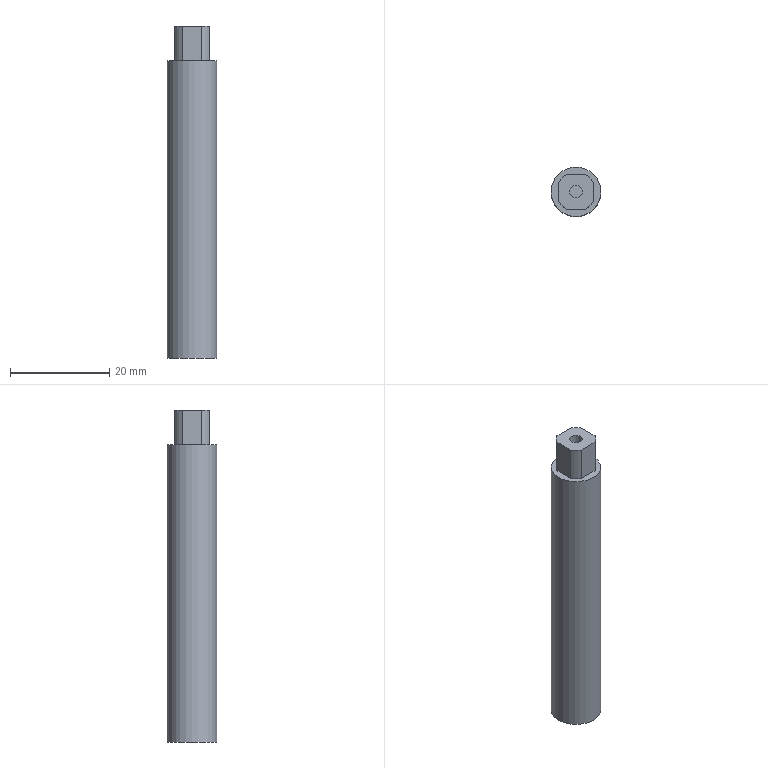Part | NX | features DATUM_CSYS 4, EXTRUDE 3, SKETCH 3 | 1 solid | 14 faces | box 10 x 10 x 67 mm | volume 4993 mm3 | plane 8 | cylinder 6 | commonest cylinder face diameters 8 x4 2.5 x1 10 x1
STEP:
#1=CARTESIAN_POINT('',(5.,0.,60.));
#2=VERTEX_POINT('',#1);
#3=CARTESIAN_POINT('',(0.,0.,60.));
#4=DIRECTION('',(0.,0.,1.));
#5=DIRECTION('',(1.,0.,0.));
#6=AXIS2_PLACEMENT_3D('',#3,#4,#5);
#7=CIRCLE('',#6,5.);
#8=EDGE_CURVE('',#2,#2,#7,.T.);
#9=ORIENTED_EDGE('',*,*,#8,.F.);
#10=EDGE_LOOP('',(#9));
#11=FACE_BOUND('',#10,.T.);
#12=CARTESIAN_POINT('',(5.,0.,0.));
#13=VERTEX_POINT('',#12);
#14=CARTESIAN_POINT('',(0.,0.,0.));
#15=DIRECTION('',(0.,0.,1.));
#16=DIRECTION('',(1.,0.,0.));
#17=AXIS2_PLACEMENT_3D('',#14,#15,#16);
#18=CIRCLE('',#17,5.);
#19=EDGE_CURVE('',#13,#13,#18,.T.);
#20=ORIENTED_EDGE('',*,*,#19,.T.);
#21=EDGE_LOOP('',(#20));
#22=FACE_BOUND('',#21,.T.);
#23=CARTESIAN_POINT('',(0.,0.,60.));
#24=DIRECTION('',(0.,0.,-1.));
#25=DIRECTION('',(-1.,0.,0.));
#26=AXIS2_PLACEMENT_3D('',#23,#24,#25);
#27=CYLINDRICAL_SURFACE('',#26,5.);
#28=ADVANCED_FACE('',(#11,#22),#27,.T.);
#29=CARTESIAN_POINT('',(-3.5,1.936,60.));
#30=VERTEX_POINT('',#29);
#31=CARTESIAN_POINT('',(-3.5,-1.936,60.));
#32=VERTEX_POINT('',#31);
#33=CARTESIAN_POINT('',(-3.5,1.936,60.));
#34=DIRECTION('',(0.,-1.,0.));
#35=VECTOR('',#34,1000.);
#36=LINE('',#33,#35);
#37=EDGE_CURVE('',#30,#32,#36,.T.);
#38=ORIENTED_EDGE('',*,*,#37,.F.);
#39=CARTESIAN_POINT('',(-1.936,3.5,60.));
#40=VERTEX_POINT('',#39);
#41=CARTESIAN_POINT('',(0.,0.,60.));
#42=DIRECTION('',(0.,0.,1.));
#43=DIRECTION('',(1.,0.,0.));
#44=AXIS2_PLACEMENT_3D('',#41,#42,#43);
#45=CIRCLE('',#44,4.);
#46=EDGE_CURVE('',#40,#30,#45,.T.);
#47=ORIENTED_EDGE('',*,*,#46,.F.);
#48=CARTESIAN_POINT('',(1.936,3.5,60.));
#49=VERTEX_POINT('',#48);
#50=CARTESIAN_POINT('',(1.936,3.5,60.));
#51=DIRECTION('',(-1.,0.,0.));
#52=VECTOR('',#51,1000.);
#53=LINE('',#50,#52);
#54=EDGE_CURVE('',#49,#40,#53,.T.);
#55=ORIENTED_EDGE('',*,*,#54,.F.);
#56=CARTESIAN_POINT('',(3.5,1.936,60.));
#57=VERTEX_POINT('',#56);
#58=CARTESIAN_POINT('',(0.,0.,60.));
#59=DIRECTION('',(0.,0.,1.));
#60=DIRECTION('',(1.,0.,0.));
#61=AXIS2_PLACEMENT_3D('',#58,#59,#60);
#62=CIRCLE('',#61,4.);
#63=EDGE_CURVE('',#57,#49,#62,.T.);
#64=ORIENTED_EDGE('',*,*,#63,.F.);
#65=CARTESIAN_POINT('',(3.5,-1.936,60.));
#66=VERTEX_POINT('',#65);
#67=CARTESIAN_POINT('',(3.5,-1.936,60.));
#68=DIRECTION('',(0.,1.,0.));
#69=VECTOR('',#68,1000.);
#70=LINE('',#67,#69);
#71=EDGE_CURVE('',#66,#57,#70,.T.);
#72=ORIENTED_EDGE('',*,*,#71,.F.);
#73=CARTESIAN_POINT('',(1.936,-3.5,60.));
#74=VERTEX_POINT('',#73);
#75=CARTESIAN_POINT('',(0.,0.,60.));
#76=DIRECTION('',(0.,0.,1.));
#77=DIRECTION('',(1.,0.,0.));
#78=AXIS2_PLACEMENT_3D('',#75,#76,#77);
#79=CIRCLE('',#78,4.);
#80=EDGE_CURVE('',#74,#66,#79,.T.);
#81=ORIENTED_EDGE('',*,*,#80,.F.);
#82=CARTESIAN_POINT('',(-1.936,-3.5,60.));
#83=VERTEX_POINT('',#82);
#84=CARTESIAN_POINT('',(-1.936,-3.5,60.));
#85=DIRECTION('',(1.,0.,0.));
#86=VECTOR('',#85,1000.);
#87=LINE('',#84,#86);
#88=EDGE_CURVE('',#83,#74,#87,.T.);
#89=ORIENTED_EDGE('',*,*,#88,.F.);
#90=CARTESIAN_POINT('',(0.,0.,60.));
#91=DIRECTION('',(0.,0.,1.));
#92=DIRECTION('',(1.,0.,0.));
#93=AXIS2_PLACEMENT_3D('',#90,#91,#92);
#94=CIRCLE('',#93,4.);
#95=EDGE_CURVE('',#32,#83,#94,.T.);
#96=ORIENTED_EDGE('',*,*,#95,.F.);
#97=EDGE_LOOP('',(#38,#47,#55,#64,#72,#81,#89,#96));
#98=FACE_BOUND('',#97,.T.);
#99=ORIENTED_EDGE('',*,*,#8,.T.);
#100=EDGE_LOOP('',(#99));
#101=FACE_BOUND('',#100,.T.);
#102=CARTESIAN_POINT('',(0.,0.,60.));
#103=DIRECTION('',(0.,0.,1.));
#104=DIRECTION('',(1.,0.,0.));
#105=AXIS2_PLACEMENT_3D('',#102,#103,#104);
#106=PLANE('',#105);
#107=ADVANCED_FACE('',(#98,#101),#106,.T.);
#108=ORIENTED_EDGE('',*,*,#19,.F.);
#109=EDGE_LOOP('',(#108));
#110=FACE_BOUND('',#109,.T.);
#111=CARTESIAN_POINT('',(0.,0.,0.));
#112=DIRECTION('',(0.,0.,1.));
#113=DIRECTION('',(1.,0.,0.));
#114=AXIS2_PLACEMENT_3D('',#111,#112,#113);
#115=PLANE('',#114);
#116=ADVANCED_FACE('',(#110),#115,.F.);
#117=ORIENTED_EDGE('',*,*,#37,.T.);
#118=CARTESIAN_POINT('',(-3.5,-1.936,67.));
#119=VERTEX_POINT('',#118);
#120=CARTESIAN_POINT('',(-3.5,-1.936,67.));
#121=DIRECTION('',(0.,0.,-1.));
#122=VECTOR('',#121,1000.);
#123=LINE('',#120,#122);
#124=EDGE_CURVE('',#119,#32,#123,.T.);
#125=ORIENTED_EDGE('',*,*,#124,.F.);
#126=CARTESIAN_POINT('',(-3.5,1.936,67.));
#127=VERTEX_POINT('',#126);
#128=CARTESIAN_POINT('',(-3.5,1.936,67.));
#129=DIRECTION('',(0.,-1.,0.));
#130=VECTOR('',#129,1000.);
#131=LINE('',#128,#130);
#132=EDGE_CURVE('',#127,#119,#131,.T.);
#133=ORIENTED_EDGE('',*,*,#132,.F.);
#134=CARTESIAN_POINT('',(-3.5,1.936,67.));
#135=DIRECTION('',(0.,0.,-1.));
#136=VECTOR('',#135,1000.);
#137=LINE('',#134,#136);
#138=EDGE_CURVE('',#127,#30,#137,.T.);
#139=ORIENTED_EDGE('',*,*,#138,.T.);
#140=EDGE_LOOP('',(#117,#125,#133,#139));
#141=FACE_BOUND('',#140,.T.);
#142=CARTESIAN_POINT('',(-3.5,1.936,67.));
#143=DIRECTION('',(1.,0.,0.));
#144=DIRECTION('',(0.,1.,0.));
#145=AXIS2_PLACEMENT_3D('',#142,#143,#144);
#146=PLANE('',#145);
#147=ADVANCED_FACE('',(#141),#146,.F.);
#148=ORIENTED_EDGE('',*,*,#95,.T.);
#149=CARTESIAN_POINT('',(-1.936,-3.5,67.));
#150=VERTEX_POINT('',#149);
#151=CARTESIAN_POINT('',(-1.936,-3.5,67.));
#152=DIRECTION('',(0.,0.,-1.));
#153=VECTOR('',#152,1000.);
#154=LINE('',#151,#153);
#155=EDGE_CURVE('',#150,#83,#154,.T.);
#156=ORIENTED_EDGE('',*,*,#155,.F.);
#157=CARTESIAN_POINT('',(0.,0.,67.));
#158=DIRECTION('',(0.,0.,1.));
#159=DIRECTION('',(1.,0.,0.));
#160=AXIS2_PLACEMENT_3D('',#157,#158,#159);
#161=CIRCLE('',#160,4.);
#162=EDGE_CURVE('',#119,#150,#161,.T.);
#163=ORIENTED_EDGE('',*,*,#162,.F.);
#164=ORIENTED_EDGE('',*,*,#124,.T.);
#165=EDGE_LOOP('',(#148,#156,#163,#164));
#166=FACE_BOUND('',#165,.T.);
#167=CARTESIAN_POINT('',(0.,0.,67.));
#168=DIRECTION('',(0.,0.,-1.));
#169=DIRECTION('',(-1.,0.,0.));
#170=AXIS2_PLACEMENT_3D('',#167,#168,#169);
#171=CYLINDRICAL_SURFACE('',#170,4.);
#172=ADVANCED_FACE('',(#166),#171,.T.);
#173=ORIENTED_EDGE('',*,*,#88,.T.);
#174=CARTESIAN_POINT('',(1.936,-3.5,67.));
#175=VERTEX_POINT('',#174);
#176=CARTESIAN_POINT('',(1.936,-3.5,67.));
#177=DIRECTION('',(0.,0.,-1.));
#178=VECTOR('',#177,1000.);
#179=LINE('',#176,#178);
#180=EDGE_CURVE('',#175,#74,#179,.T.);
#181=ORIENTED_EDGE('',*,*,#180,.F.);
#182=CARTESIAN_POINT('',(-1.936,-3.5,67.));
#183=DIRECTION('',(1.,0.,0.));
#184=VECTOR('',#183,1000.);
#185=LINE('',#182,#184);
#186=EDGE_CURVE('',#150,#175,#185,.T.);
#187=ORIENTED_EDGE('',*,*,#186,.F.);
#188=ORIENTED_EDGE('',*,*,#155,.T.);
#189=EDGE_LOOP('',(#173,#181,#187,#188));
#190=FACE_BOUND('',#189,.T.);
#191=CARTESIAN_POINT('',(-1.936,-3.5,67.));
#192=DIRECTION('',(0.,1.,0.));
#193=DIRECTION('',(0.,0.,1.));
#194=AXIS2_PLACEMENT_3D('',#191,#192,#193);
#195=PLANE('',#194);
#196=ADVANCED_FACE('',(#190),#195,.F.);
#197=ORIENTED_EDGE('',*,*,#80,.T.);
#198=CARTESIAN_POINT('',(3.5,-1.936,67.));
#199=VERTEX_POINT('',#198);
#200=CARTESIAN_POINT('',(3.5,-1.936,67.));
#201=DIRECTION('',(0.,0.,-1.));
#202=VECTOR('',#201,1000.);
#203=LINE('',#200,#202);
#204=EDGE_CURVE('',#199,#66,#203,.T.);
#205=ORIENTED_EDGE('',*,*,#204,.F.);
#206=CARTESIAN_POINT('',(0.,0.,67.));
#207=DIRECTION('',(0.,0.,1.));
#208=DIRECTION('',(1.,0.,0.));
#209=AXIS2_PLACEMENT_3D('',#206,#207,#208);
#210=CIRCLE('',#209,4.);
#211=EDGE_CURVE('',#175,#199,#210,.T.);
#212=ORIENTED_EDGE('',*,*,#211,.F.);
#213=ORIENTED_EDGE('',*,*,#180,.T.);
#214=EDGE_LOOP('',(#197,#205,#212,#213));
#215=FACE_BOUND('',#214,.T.);
#216=CARTESIAN_POINT('',(0.,0.,67.));
#217=DIRECTION('',(0.,0.,-1.));
#218=DIRECTION('',(-1.,0.,0.));
#219=AXIS2_PLACEMENT_3D('',#216,#217,#218);
#220=CYLINDRICAL_SURFACE('',#219,4.);
#221=ADVANCED_FACE('',(#215),#220,.T.);
#222=ORIENTED_EDGE('',*,*,#71,.T.);
#223=CARTESIAN_POINT('',(3.5,1.936,67.));
#224=VERTEX_POINT('',#223);
#225=CARTESIAN_POINT('',(3.5,1.936,67.));
#226=DIRECTION('',(0.,0.,-1.));
#227=VECTOR('',#226,1000.);
#228=LINE('',#225,#227);
#229=EDGE_CURVE('',#224,#57,#228,.T.);
#230=ORIENTED_EDGE('',*,*,#229,.F.);
#231=CARTESIAN_POINT('',(3.5,-1.936,67.));
#232=DIRECTION('',(0.,1.,0.));
#233=VECTOR('',#232,1000.);
#234=LINE('',#231,#233);
#235=EDGE_CURVE('',#199,#224,#234,.T.);
#236=ORIENTED_EDGE('',*,*,#235,.F.);
#237=ORIENTED_EDGE('',*,*,#204,.T.);
#238=EDGE_LOOP('',(#222,#230,#236,#237));
#239=FACE_BOUND('',#238,.T.);
#240=CARTESIAN_POINT('',(3.5,-1.936,67.));
#241=DIRECTION('',(-1.,0.,0.));
#242=DIRECTION('',(0.,-1.,0.));
#243=AXIS2_PLACEMENT_3D('',#240,#241,#242);
#244=PLANE('',#243);
#245=ADVANCED_FACE('',(#239),#244,.F.);
#246=ORIENTED_EDGE('',*,*,#63,.T.);
#247=CARTESIAN_POINT('',(1.936,3.5,67.));
#248=VERTEX_POINT('',#247);
#249=CARTESIAN_POINT('',(1.936,3.5,67.));
#250=DIRECTION('',(0.,0.,-1.));
#251=VECTOR('',#250,1000.);
#252=LINE('',#249,#251);
#253=EDGE_CURVE('',#248,#49,#252,.T.);
#254=ORIENTED_EDGE('',*,*,#253,.F.);
#255=CARTESIAN_POINT('',(0.,0.,67.));
#256=DIRECTION('',(0.,0.,1.));
#257=DIRECTION('',(1.,0.,0.));
#258=AXIS2_PLACEMENT_3D('',#255,#256,#257);
#259=CIRCLE('',#258,4.);
#260=EDGE_CURVE('',#224,#248,#259,.T.);
#261=ORIENTED_EDGE('',*,*,#260,.F.);
#262=ORIENTED_EDGE('',*,*,#229,.T.);
#263=EDGE_LOOP('',(#246,#254,#261,#262));
#264=FACE_BOUND('',#263,.T.);
#265=CARTESIAN_POINT('',(0.,0.,67.));
#266=DIRECTION('',(0.,0.,-1.));
#267=DIRECTION('',(-1.,0.,0.));
#268=AXIS2_PLACEMENT_3D('',#265,#266,#267);
#269=CYLINDRICAL_SURFACE('',#268,4.);
#270=ADVANCED_FACE('',(#264),#269,.T.);
#271=ORIENTED_EDGE('',*,*,#54,.T.);
#272=CARTESIAN_POINT('',(-1.936,3.5,67.));
#273=VERTEX_POINT('',#272);
#274=CARTESIAN_POINT('',(-1.936,3.5,67.));
#275=DIRECTION('',(0.,0.,-1.));
#276=VECTOR('',#275,1000.);
#277=LINE('',#274,#276);
#278=EDGE_CURVE('',#273,#40,#277,.T.);
#279=ORIENTED_EDGE('',*,*,#278,.F.);
#280=CARTESIAN_POINT('',(1.936,3.5,67.));
#281=DIRECTION('',(-1.,0.,0.));
#282=VECTOR('',#281,1000.);
#283=LINE('',#280,#282);
#284=EDGE_CURVE('',#248,#273,#283,.T.);
#285=ORIENTED_EDGE('',*,*,#284,.F.);
#286=ORIENTED_EDGE('',*,*,#253,.T.);
#287=EDGE_LOOP('',(#271,#279,#285,#286));
#288=FACE_BOUND('',#287,.T.);
#289=CARTESIAN_POINT('',(1.936,3.5,67.));
#290=DIRECTION('',(0.,-1.,0.));
#291=DIRECTION('',(0.,0.,-1.));
#292=AXIS2_PLACEMENT_3D('',#289,#290,#291);
#293=PLANE('',#292);
#294=ADVANCED_FACE('',(#288),#293,.F.);
#295=ORIENTED_EDGE('',*,*,#46,.T.);
#296=ORIENTED_EDGE('',*,*,#138,.F.);
#297=CARTESIAN_POINT('',(0.,0.,67.));
#298=DIRECTION('',(0.,0.,1.));
#299=DIRECTION('',(1.,0.,0.));
#300=AXIS2_PLACEMENT_3D('',#297,#298,#299);
#301=CIRCLE('',#300,4.);
#302=EDGE_CURVE('',#273,#127,#301,.T.);
#303=ORIENTED_EDGE('',*,*,#302,.F.);
#304=ORIENTED_EDGE('',*,*,#278,.T.);
#305=EDGE_LOOP('',(#295,#296,#303,#304));
#306=FACE_BOUND('',#305,.T.);
#307=CARTESIAN_POINT('',(0.,0.,67.));
#308=DIRECTION('',(0.,0.,-1.));
#309=DIRECTION('',(-1.,0.,0.));
#310=AXIS2_PLACEMENT_3D('',#307,#308,#309);
#311=CYLINDRICAL_SURFACE('',#310,4.);
#312=ADVANCED_FACE('',(#306),#311,.T.);
#313=CARTESIAN_POINT('',(1.25,0.,67.));
#314=VERTEX_POINT('',#313);
#315=CARTESIAN_POINT('',(0.,0.,67.));
#316=DIRECTION('',(0.,0.,1.));
#317=DIRECTION('',(1.,0.,0.));
#318=AXIS2_PLACEMENT_3D('',#315,#316,#317);
#319=CIRCLE('',#318,1.25);
#320=EDGE_CURVE('',#314,#314,#319,.T.);
#321=ORIENTED_EDGE('',*,*,#320,.F.);
#322=EDGE_LOOP('',(#321));
#323=FACE_BOUND('',#322,.T.);
#324=ORIENTED_EDGE('',*,*,#132,.T.);
#325=ORIENTED_EDGE('',*,*,#162,.T.);
#326=ORIENTED_EDGE('',*,*,#186,.T.);
#327=ORIENTED_EDGE('',*,*,#211,.T.);
#328=ORIENTED_EDGE('',*,*,#235,.T.);
#329=ORIENTED_EDGE('',*,*,#260,.T.);
#330=ORIENTED_EDGE('',*,*,#284,.T.);
#331=ORIENTED_EDGE('',*,*,#302,.T.);
#332=EDGE_LOOP('',(#324,#325,#326,#327,#328,#329,#330,#331));
#333=FACE_BOUND('',#332,.T.);
#334=CARTESIAN_POINT('',(0.,0.,67.));
#335=DIRECTION('',(0.,0.,1.));
#336=DIRECTION('',(1.,0.,0.));
#337=AXIS2_PLACEMENT_3D('',#334,#335,#336);
#338=PLANE('',#337);
#339=ADVANCED_FACE('',(#323,#333),#338,.T.);
#340=CARTESIAN_POINT('',(1.25,0.,60.));
#341=VERTEX_POINT('',#340);
#342=CARTESIAN_POINT('',(0.,0.,60.));
#343=DIRECTION('',(0.,0.,1.));
#344=DIRECTION('',(1.,0.,0.));
#345=AXIS2_PLACEMENT_3D('',#342,#343,#344);
#346=CIRCLE('',#345,1.25);
#347=EDGE_CURVE('',#341,#341,#346,.F.);
#348=ORIENTED_EDGE('',*,*,#347,.T.);
#349=EDGE_LOOP('',(#348));
#350=FACE_BOUND('',#349,.T.);
#351=ORIENTED_EDGE('',*,*,#320,.T.);
#352=EDGE_LOOP('',(#351));
#353=FACE_BOUND('',#352,.T.);
#354=CARTESIAN_POINT('',(0.,0.,60.));
#355=DIRECTION('',(0.,0.,1.));
#356=DIRECTION('',(1.,0.,0.));
#357=AXIS2_PLACEMENT_3D('',#354,#355,#356);
#358=CYLINDRICAL_SURFACE('',#357,1.25);
#359=ADVANCED_FACE('',(#350,#353),#358,.F.);
#360=ORIENTED_EDGE('',*,*,#347,.F.);
#361=EDGE_LOOP('',(#360));
#362=FACE_BOUND('',#361,.T.);
#363=CARTESIAN_POINT('',(0.,0.,60.));
#364=DIRECTION('',(0.,0.,1.));
#365=DIRECTION('',(1.,0.,0.));
#366=AXIS2_PLACEMENT_3D('',#363,#364,#365);
#367=PLANE('',#366);
#368=ADVANCED_FACE('',(#362),#367,.T.);
#369=CLOSED_SHELL('',(#28,#107,#116,#147,#172,#196,#221,#245,#270,#294,#312,#339,#359,#368));
#370=MANIFOLD_SOLID_BREP('',#369);
#371=(LENGTH_UNIT()NAMED_UNIT(*)SI_UNIT(.MILLI.,.METRE.));
#372=UNCERTAINTY_MEASURE_WITH_UNIT(LENGTH_MEASURE(0.00001),#371,'','');
#373=(NAMED_UNIT(*)PLANE_ANGLE_UNIT()SI_UNIT($,.RADIAN.));
#374=(NAMED_UNIT(*)SI_UNIT($,.STERADIAN.)SOLID_ANGLE_UNIT());
#375=(GEOMETRIC_REPRESENTATION_CONTEXT(3)GLOBAL_UNCERTAINTY_ASSIGNED_CONTEXT((#372))GLOBAL_UNIT_ASSIGNED_CONTEXT((#371,#373,#374))REPRESENTATION_CONTEXT('',''));
#376=ADVANCED_BREP_SHAPE_REPRESENTATION('',(#370),#375);